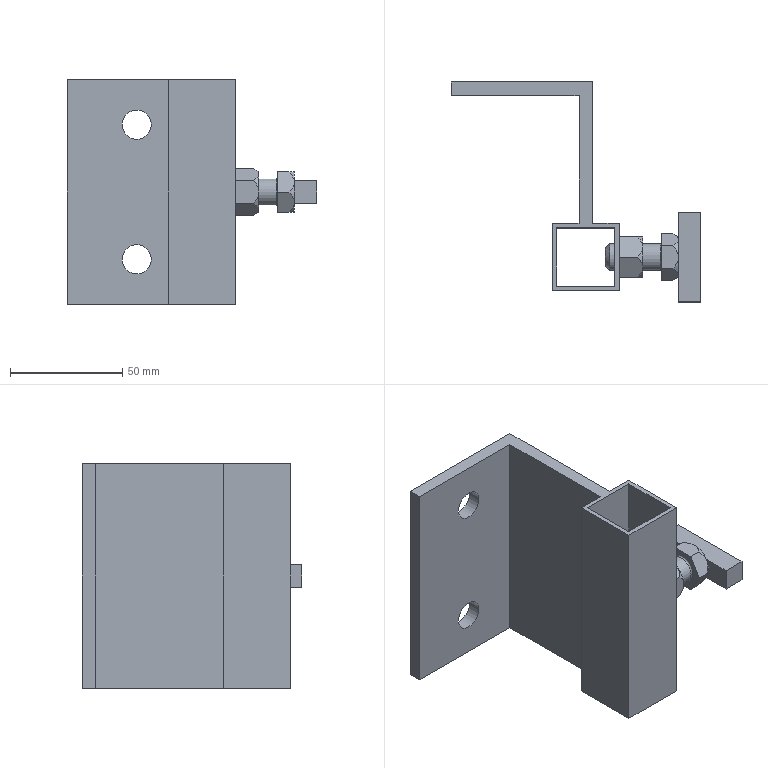Part | NX | features solid 2 | 1 solid | 62 faces | box 111.3 x 98 x 100 mm | volume 103165 mm3 | plane 41 | cone 15 | cylinder 5 | torus 1 | commonest cylinder face diameters 12 x3 13 x2